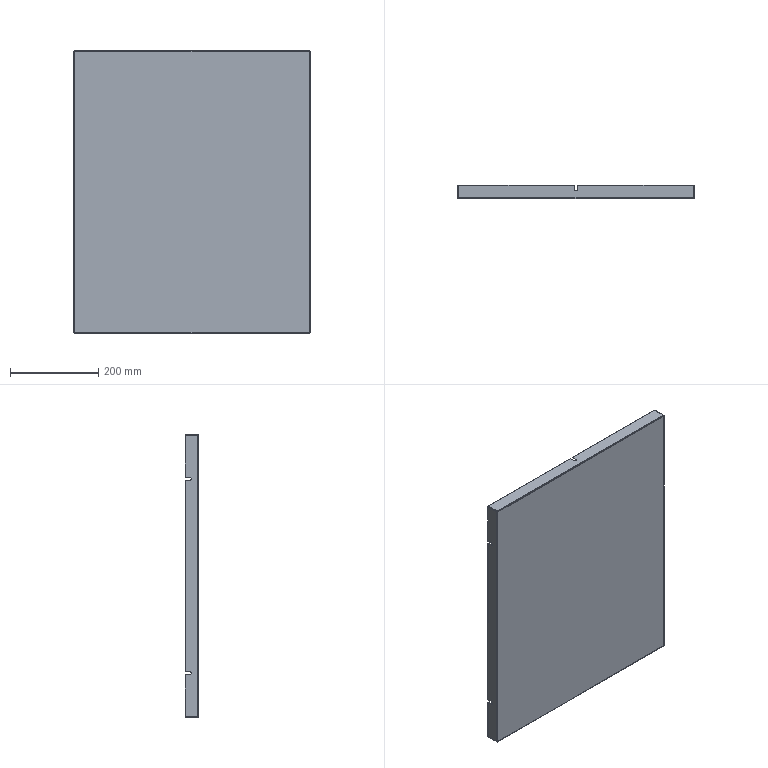Part | STEP file | JBJ-P-1011-06 | 1 solid | 62 faces | box 535 x 30 x 640 mm | volume 489037 mm3 | plane 40 | cylinder 14 | spline 8 | commonest cylinder face diameters 6.5 x6 2 x4 4.4 x4